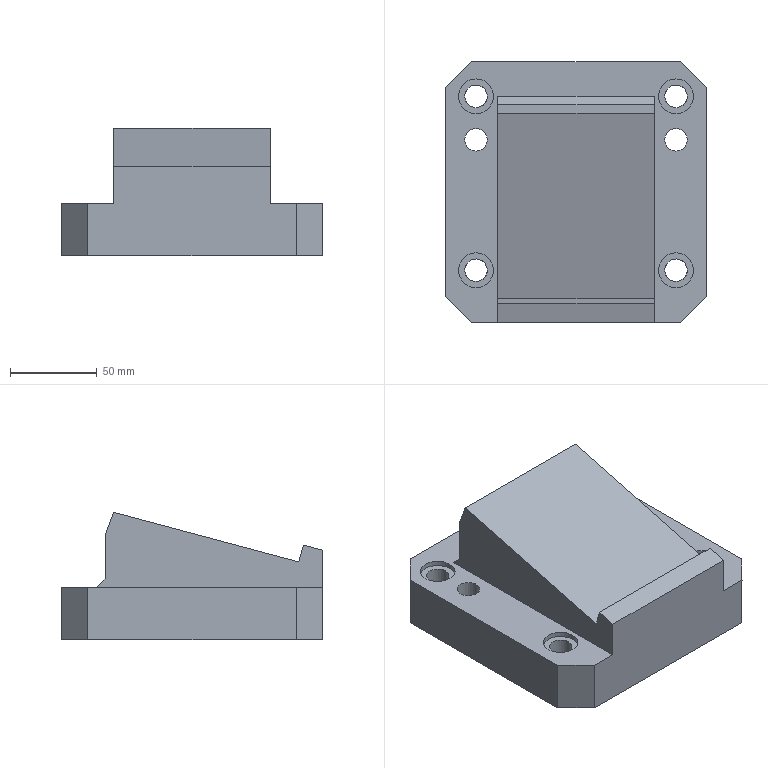Part | NX | features solid 2 | 1 solid | 41 faces | box 150 x 150 x 73.352 mm | volume 930755 mm3 | plane 31 | cylinder 10 | commonest cylinder face diameters 13 x6 20 x4
STEP:
#1=CARTESIAN_POINT('',(227.5,985.,-285.));
#2=VERTEX_POINT('',#1);
#3=CARTESIAN_POINT('',(227.5,995.,-285.));
#4=DIRECTION('',(0.,0.000000003,-1.));
#5=DIRECTION('',(0.,-1.,-0.000000003));
#6=AXIS2_PLACEMENT_3D('',#3,#4,#5);
#7=CIRCLE('',#6,10.);
#8=EDGE_CURVE('',#2,#2,#7,.T.);
#9=ORIENTED_EDGE('',*,*,#8,.T.);
#10=EDGE_LOOP('',(#9));
#11=FACE_BOUND('',#10,.T.);
#12=CARTESIAN_POINT('',(227.5,885.,-285.));
#13=VERTEX_POINT('',#12);
#14=CARTESIAN_POINT('',(227.5,895.,-285.));
#15=DIRECTION('',(0.,0.000000003,-1.));
#16=DIRECTION('',(0.,-1.,-0.000000003));
#17=AXIS2_PLACEMENT_3D('',#14,#15,#16);
#18=CIRCLE('',#17,10.);
#19=EDGE_CURVE('',#13,#13,#18,.T.);
#20=ORIENTED_EDGE('',*,*,#19,.T.);
#21=EDGE_LOOP('',(#20));
#22=FACE_BOUND('',#21,.T.);
#23=CARTESIAN_POINT('',(112.5,963.5,-285.));
#24=VERTEX_POINT('',#23);
#25=CARTESIAN_POINT('',(112.5,970.,-285.));
#26=DIRECTION('',(0.,0.000000003,-1.));
#27=DIRECTION('',(0.,-1.,-0.000000003));
#28=AXIS2_PLACEMENT_3D('',#25,#26,#27);
#29=CIRCLE('',#28,6.5);
#30=EDGE_CURVE('',#24,#24,#29,.T.);
#31=ORIENTED_EDGE('',*,*,#30,.T.);
#32=EDGE_LOOP('',(#31));
#33=FACE_BOUND('',#32,.T.);
#34=CARTESIAN_POINT('',(227.5,963.5,-285.));
#35=VERTEX_POINT('',#34);
#36=CARTESIAN_POINT('',(227.5,970.,-285.));
#37=DIRECTION('',(0.,0.000000003,-1.));
#38=DIRECTION('',(0.,-1.,-0.000000003));
#39=AXIS2_PLACEMENT_3D('',#36,#37,#38);
#40=CIRCLE('',#39,6.5);
#41=EDGE_CURVE('',#35,#35,#40,.T.);
#42=ORIENTED_EDGE('',*,*,#41,.T.);
#43=EDGE_LOOP('',(#42));
#44=FACE_BOUND('',#43,.T.);
#45=CARTESIAN_POINT('',(112.5,885.,-285.));
#46=VERTEX_POINT('',#45);
#47=CARTESIAN_POINT('',(112.5,895.,-285.));
#48=DIRECTION('',(0.,0.000000003,-1.));
#49=DIRECTION('',(0.,-1.,-0.000000003));
#50=AXIS2_PLACEMENT_3D('',#47,#48,#49);
#51=CIRCLE('',#50,10.);
#52=EDGE_CURVE('',#46,#46,#51,.T.);
#53=ORIENTED_EDGE('',*,*,#52,.T.);
#54=EDGE_LOOP('',(#53));
#55=FACE_BOUND('',#54,.T.);
#56=CARTESIAN_POINT('',(112.5,985.,-285.));
#57=VERTEX_POINT('',#56);
#58=CARTESIAN_POINT('',(112.5,995.,-285.));
#59=DIRECTION('',(0.,0.000000003,-1.));
#60=DIRECTION('',(0.,-1.,-0.000000003));
#61=AXIS2_PLACEMENT_3D('',#58,#59,#60);
#62=CIRCLE('',#61,10.);
#63=EDGE_CURVE('',#57,#57,#62,.T.);
#64=ORIENTED_EDGE('',*,*,#63,.T.);
#65=EDGE_LOOP('',(#64));
#66=FACE_BOUND('',#65,.T.);
#67=CARTESIAN_POINT('',(215.,995.,-285.));
#68=VERTEX_POINT('',#67);
#69=CARTESIAN_POINT('',(215.,865.,-285.));
#70=VERTEX_POINT('',#69);
#71=CARTESIAN_POINT('',(215.,990.,-285.));
#72=DIRECTION('',(0.,-1.,-0.000000003));
#73=VECTOR('',#72,1000.);
#74=LINE('',#71,#73);
#75=EDGE_CURVE('',#68,#70,#74,.T.);
#76=ORIENTED_EDGE('',*,*,#75,.T.);
#77=CARTESIAN_POINT('',(230.,865.,-285.));
#78=VERTEX_POINT('',#77);
#79=CARTESIAN_POINT('',(110.,865.,-285.));
#80=DIRECTION('',(1.,0.,0.));
#81=VECTOR('',#80,1000.);
#82=LINE('',#79,#81);
#83=EDGE_CURVE('',#70,#78,#82,.T.);
#84=ORIENTED_EDGE('',*,*,#83,.T.);
#85=CARTESIAN_POINT('',(245.,880.,-285.));
#86=VERTEX_POINT('',#85);
#87=CARTESIAN_POINT('',(245.,880.,-285.));
#88=DIRECTION('',(-0.7071,-0.7071,-0.000000002));
#89=VECTOR('',#88,1000.);
#90=LINE('',#87,#89);
#91=EDGE_CURVE('',#86,#78,#90,.T.);
#92=ORIENTED_EDGE('',*,*,#91,.F.);
#93=CARTESIAN_POINT('',(245.,1000.,-285.));
#94=VERTEX_POINT('',#93);
#95=CARTESIAN_POINT('',(245.,1000.,-285.));
#96=DIRECTION('',(0.,-1.,-0.000000003));
#97=VECTOR('',#96,1000.);
#98=LINE('',#95,#97);
#99=EDGE_CURVE('',#94,#86,#98,.T.);
#100=ORIENTED_EDGE('',*,*,#99,.F.);
#101=CARTESIAN_POINT('',(230.,1015.,-285.));
#102=VERTEX_POINT('',#101);
#103=CARTESIAN_POINT('',(230.,1015.,-285.));
#104=DIRECTION('',(0.7071,-0.7071,-0.000000002));
#105=VECTOR('',#104,1000.);
#106=LINE('',#103,#105);
#107=EDGE_CURVE('',#102,#94,#106,.T.);
#108=ORIENTED_EDGE('',*,*,#107,.F.);
#109=CARTESIAN_POINT('',(110.,1015.,-285.));
#110=VERTEX_POINT('',#109);
#111=CARTESIAN_POINT('',(110.,1015.,-285.));
#112=DIRECTION('',(1.,0.,0.));
#113=VECTOR('',#112,1000.);
#114=LINE('',#111,#113);
#115=EDGE_CURVE('',#110,#102,#114,.T.);
#116=ORIENTED_EDGE('',*,*,#115,.F.);
#117=CARTESIAN_POINT('',(95.,1000.,-285.));
#118=VERTEX_POINT('',#117);
#119=CARTESIAN_POINT('',(95.,1000.,-285.));
#120=DIRECTION('',(0.7071,0.7071,0.000000002));
#121=VECTOR('',#120,1000.);
#122=LINE('',#119,#121);
#123=EDGE_CURVE('',#118,#110,#122,.T.);
#124=ORIENTED_EDGE('',*,*,#123,.F.);
#125=CARTESIAN_POINT('',(95.,880.,-285.));
#126=VERTEX_POINT('',#125);
#127=CARTESIAN_POINT('',(95.,1000.,-285.));
#128=DIRECTION('',(0.,-1.,-0.000000003));
#129=VECTOR('',#128,1000.);
#130=LINE('',#127,#129);
#131=EDGE_CURVE('',#118,#126,#130,.T.);
#132=ORIENTED_EDGE('',*,*,#131,.T.);
#133=CARTESIAN_POINT('',(110.,865.,-285.));
#134=VERTEX_POINT('',#133);
#135=CARTESIAN_POINT('',(110.,865.,-285.));
#136=DIRECTION('',(-0.7071,0.7071,0.000000002));
#137=VECTOR('',#136,1000.);
#138=LINE('',#135,#137);
#139=EDGE_CURVE('',#134,#126,#138,.T.);
#140=ORIENTED_EDGE('',*,*,#139,.F.);
#141=CARTESIAN_POINT('',(125.,865.,-285.));
#142=VERTEX_POINT('',#141);
#143=CARTESIAN_POINT('',(110.,865.,-285.));
#144=DIRECTION('',(1.,0.,0.));
#145=VECTOR('',#144,1000.);
#146=LINE('',#143,#145);
#147=EDGE_CURVE('',#134,#142,#146,.T.);
#148=ORIENTED_EDGE('',*,*,#147,.T.);
#149=CARTESIAN_POINT('',(125.,995.,-285.));
#150=VERTEX_POINT('',#149);
#151=CARTESIAN_POINT('',(125.,990.,-285.));
#152=DIRECTION('',(0.,-1.,-0.000000003));
#153=VECTOR('',#152,1000.);
#154=LINE('',#151,#153);
#155=EDGE_CURVE('',#150,#142,#154,.T.);
#156=ORIENTED_EDGE('',*,*,#155,.F.);
#157=CARTESIAN_POINT('',(170.,995.,-285.));
#158=DIRECTION('',(-1.,0.,0.));
#159=VECTOR('',#158,1000.);
#160=LINE('',#157,#159);
#161=EDGE_CURVE('',#68,#150,#160,.T.);
#162=ORIENTED_EDGE('',*,*,#161,.F.);
#163=EDGE_LOOP('',(#76,#84,#92,#100,#108,#116,#124,#132,#140,#148,#156,#162));
#164=FACE_BOUND('',#163,.T.);
#165=CARTESIAN_POINT('',(170.,805.,-285.));
#166=DIRECTION('',(0.,0.000000003,-1.));
#167=DIRECTION('',(-1.,0.,0.));
#168=AXIS2_PLACEMENT_3D('',#165,#166,#167);
#169=PLANE('',#168);
#170=ADVANCED_FACE('',(#11,#22,#33,#44,#55,#66,#164),#169,.F.);
#171=CARTESIAN_POINT('',(227.5,988.5,-315.));
#172=VERTEX_POINT('',#171);
#173=CARTESIAN_POINT('',(227.5,995.,-315.));
#174=DIRECTION('',(0.,0.000000003,-1.));
#175=DIRECTION('',(0.,-1.,-0.000000003));
#176=AXIS2_PLACEMENT_3D('',#173,#174,#175);
#177=CIRCLE('',#176,6.5);
#178=EDGE_CURVE('',#172,#172,#177,.T.);
#179=ORIENTED_EDGE('',*,*,#178,.T.);
#180=EDGE_LOOP('',(#179));
#181=FACE_BOUND('',#180,.T.);
#182=CARTESIAN_POINT('',(234.,995.,-288.));
#183=VERTEX_POINT('',#182);
#184=CARTESIAN_POINT('',(227.5,995.,-288.));
#185=DIRECTION('',(0.,0.000000003,-1.));
#186=DIRECTION('',(1.,0.,0.));
#187=AXIS2_PLACEMENT_3D('',#184,#185,#186);
#188=CIRCLE('',#187,6.5);
#189=EDGE_CURVE('',#183,#183,#188,.T.);
#190=ORIENTED_EDGE('',*,*,#189,.F.);
#191=EDGE_LOOP('',(#190));
#192=FACE_BOUND('',#191,.T.);
#193=CARTESIAN_POINT('',(227.5,995.,-285.));
#194=DIRECTION('',(0.,0.000000003,-1.));
#195=DIRECTION('',(-1.,0.,0.));
#196=AXIS2_PLACEMENT_3D('',#193,#194,#195);
#197=CYLINDRICAL_SURFACE('',#196,6.5);
#198=ADVANCED_FACE('',(#181,#192),#197,.F.);
#199=CARTESIAN_POINT('',(112.5,988.5,-315.));
#200=VERTEX_POINT('',#199);
#201=CARTESIAN_POINT('',(112.5,995.,-315.));
#202=DIRECTION('',(0.,0.000000003,-1.));
#203=DIRECTION('',(0.,-1.,-0.000000003));
#204=AXIS2_PLACEMENT_3D('',#201,#202,#203);
#205=CIRCLE('',#204,6.5);
#206=EDGE_CURVE('',#200,#200,#205,.T.);
#207=ORIENTED_EDGE('',*,*,#206,.T.);
#208=EDGE_LOOP('',(#207));
#209=FACE_BOUND('',#208,.T.);
#210=CARTESIAN_POINT('',(119.,995.,-288.));
#211=VERTEX_POINT('',#210);
#212=CARTESIAN_POINT('',(112.5,995.,-288.));
#213=DIRECTION('',(0.,0.000000003,-1.));
#214=DIRECTION('',(1.,0.,0.));
#215=AXIS2_PLACEMENT_3D('',#212,#213,#214);
#216=CIRCLE('',#215,6.5);
#217=EDGE_CURVE('',#211,#211,#216,.T.);
#218=ORIENTED_EDGE('',*,*,#217,.F.);
#219=EDGE_LOOP('',(#218));
#220=FACE_BOUND('',#219,.T.);
#221=CARTESIAN_POINT('',(112.5,995.,-285.));
#222=DIRECTION('',(0.,0.000000003,-1.));
#223=DIRECTION('',(-1.,0.,0.));
#224=AXIS2_PLACEMENT_3D('',#221,#222,#223);
#225=CYLINDRICAL_SURFACE('',#224,6.5);
#226=ADVANCED_FACE('',(#209,#220),#225,.F.);
#227=CARTESIAN_POINT('',(227.5,888.5,-315.));
#228=VERTEX_POINT('',#227);
#229=CARTESIAN_POINT('',(227.5,895.,-315.));
#230=DIRECTION('',(0.,0.000000003,-1.));
#231=DIRECTION('',(0.,-1.,-0.000000003));
#232=AXIS2_PLACEMENT_3D('',#229,#230,#231);
#233=CIRCLE('',#232,6.5);
#234=EDGE_CURVE('',#228,#228,#233,.T.);
#235=ORIENTED_EDGE('',*,*,#234,.T.);
#236=EDGE_LOOP('',(#235));
#237=FACE_BOUND('',#236,.T.);
#238=CARTESIAN_POINT('',(234.,895.,-288.));
#239=VERTEX_POINT('',#238);
#240=CARTESIAN_POINT('',(227.5,895.,-288.));
#241=DIRECTION('',(0.,0.000000003,-1.));
#242=DIRECTION('',(1.,0.,0.));
#243=AXIS2_PLACEMENT_3D('',#240,#241,#242);
#244=CIRCLE('',#243,6.5);
#245=EDGE_CURVE('',#239,#239,#244,.T.);
#246=ORIENTED_EDGE('',*,*,#245,.F.);
#247=EDGE_LOOP('',(#246));
#248=FACE_BOUND('',#247,.T.);
#249=CARTESIAN_POINT('',(227.5,895.,-285.));
#250=DIRECTION('',(0.,0.000000003,-1.));
#251=DIRECTION('',(-1.,0.,0.));
#252=AXIS2_PLACEMENT_3D('',#249,#250,#251);
#253=CYLINDRICAL_SURFACE('',#252,6.5);
#254=ADVANCED_FACE('',(#237,#248),#253,.F.);
#255=CARTESIAN_POINT('',(112.5,888.5,-315.));
#256=VERTEX_POINT('',#255);
#257=CARTESIAN_POINT('',(112.5,895.,-315.));
#258=DIRECTION('',(0.,0.000000003,-1.));
#259=DIRECTION('',(0.,-1.,-0.000000003));
#260=AXIS2_PLACEMENT_3D('',#257,#258,#259);
#261=CIRCLE('',#260,6.5);
#262=EDGE_CURVE('',#256,#256,#261,.T.);
#263=ORIENTED_EDGE('',*,*,#262,.T.);
#264=EDGE_LOOP('',(#263));
#265=FACE_BOUND('',#264,.T.);
#266=CARTESIAN_POINT('',(119.,895.,-288.));
#267=VERTEX_POINT('',#266);
#268=CARTESIAN_POINT('',(112.5,895.,-288.));
#269=DIRECTION('',(0.,0.000000003,-1.));
#270=DIRECTION('',(1.,0.,0.));
#271=AXIS2_PLACEMENT_3D('',#268,#269,#270);
#272=CIRCLE('',#271,6.5);
#273=EDGE_CURVE('',#267,#267,#272,.T.);
#274=ORIENTED_EDGE('',*,*,#273,.F.);
#275=EDGE_LOOP('',(#274));
#276=FACE_BOUND('',#275,.T.);
#277=CARTESIAN_POINT('',(112.5,895.,-285.));
#278=DIRECTION('',(0.,0.000000003,-1.));
#279=DIRECTION('',(-1.,0.,0.));
#280=AXIS2_PLACEMENT_3D('',#277,#278,#279);
#281=CYLINDRICAL_SURFACE('',#280,6.5);
#282=ADVANCED_FACE('',(#265,#276),#281,.F.);
#283=CARTESIAN_POINT('',(227.5,963.5,-315.));
#284=VERTEX_POINT('',#283);
#285=CARTESIAN_POINT('',(227.5,970.,-315.));
#286=DIRECTION('',(0.,0.000000003,-1.));
#287=DIRECTION('',(0.,-1.,-0.000000003));
#288=AXIS2_PLACEMENT_3D('',#285,#286,#287);
#289=CIRCLE('',#288,6.5);
#290=EDGE_CURVE('',#284,#284,#289,.T.);
#291=ORIENTED_EDGE('',*,*,#290,.F.);
#292=EDGE_LOOP('',(#291));
#293=FACE_BOUND('',#292,.T.);
#294=ORIENTED_EDGE('',*,*,#206,.F.);
#295=EDGE_LOOP('',(#294));
#296=FACE_BOUND('',#295,.T.);
#297=ORIENTED_EDGE('',*,*,#262,.F.);
#298=EDGE_LOOP('',(#297));
#299=FACE_BOUND('',#298,.T.);
#300=CARTESIAN_POINT('',(110.,865.,-315.));
#301=VERTEX_POINT('',#300);
#302=CARTESIAN_POINT('',(95.,880.,-315.));
#303=VERTEX_POINT('',#302);
#304=CARTESIAN_POINT('',(110.,865.,-315.));
#305=DIRECTION('',(-0.7071,0.7071,0.000000002));
#306=VECTOR('',#305,1000.);
#307=LINE('',#304,#306);
#308=EDGE_CURVE('',#301,#303,#307,.T.);
#309=ORIENTED_EDGE('',*,*,#308,.T.);
#310=CARTESIAN_POINT('',(95.,1000.,-315.));
#311=VERTEX_POINT('',#310);
#312=CARTESIAN_POINT('',(95.,1000.,-315.));
#313=DIRECTION('',(0.,-1.,-0.000000003));
#314=VECTOR('',#313,1000.);
#315=LINE('',#312,#314);
#316=EDGE_CURVE('',#311,#303,#315,.T.);
#317=ORIENTED_EDGE('',*,*,#316,.F.);
#318=CARTESIAN_POINT('',(110.,1015.,-315.));
#319=VERTEX_POINT('',#318);
#320=CARTESIAN_POINT('',(95.,1000.,-315.));
#321=DIRECTION('',(0.7071,0.7071,0.000000002));
#322=VECTOR('',#321,1000.);
#323=LINE('',#320,#322);
#324=EDGE_CURVE('',#311,#319,#323,.T.);
#325=ORIENTED_EDGE('',*,*,#324,.T.);
#326=CARTESIAN_POINT('',(230.,1015.,-315.));
#327=VERTEX_POINT('',#326);
#328=CARTESIAN_POINT('',(110.,1015.,-315.));
#329=DIRECTION('',(1.,0.,0.));
#330=VECTOR('',#329,1000.);
#331=LINE('',#328,#330);
#332=EDGE_CURVE('',#319,#327,#331,.T.);
#333=ORIENTED_EDGE('',*,*,#332,.T.);
#334=CARTESIAN_POINT('',(245.,1000.,-315.));
#335=VERTEX_POINT('',#334);
#336=CARTESIAN_POINT('',(230.,1015.,-315.));
#337=DIRECTION('',(0.7071,-0.7071,-0.000000002));
#338=VECTOR('',#337,1000.);
#339=LINE('',#336,#338);
#340=EDGE_CURVE('',#327,#335,#339,.T.);
#341=ORIENTED_EDGE('',*,*,#340,.T.);
#342=CARTESIAN_POINT('',(245.,880.,-315.));
#343=VERTEX_POINT('',#342);
#344=CARTESIAN_POINT('',(245.,1000.,-315.));
#345=DIRECTION('',(0.,-1.,-0.000000003));
#346=VECTOR('',#345,1000.);
#347=LINE('',#344,#346);
#348=EDGE_CURVE('',#335,#343,#347,.T.);
#349=ORIENTED_EDGE('',*,*,#348,.T.);
#350=CARTESIAN_POINT('',(230.,865.,-315.));
#351=VERTEX_POINT('',#350);
#352=CARTESIAN_POINT('',(245.,880.,-315.));
#353=DIRECTION('',(-0.7071,-0.7071,-0.000000002));
#354=VECTOR('',#353,1000.);
#355=LINE('',#352,#354);
#356=EDGE_CURVE('',#343,#351,#355,.T.);
#357=ORIENTED_EDGE('',*,*,#356,.T.);
#358=CARTESIAN_POINT('',(110.,865.,-315.));
#359=DIRECTION('',(1.,0.,0.));
#360=VECTOR('',#359,1000.);
#361=LINE('',#358,#360);
#362=EDGE_CURVE('',#301,#351,#361,.T.);
#363=ORIENTED_EDGE('',*,*,#362,.F.);
#364=EDGE_LOOP('',(#309,#317,#325,#333,#341,#349,#357,#363));
#365=FACE_BOUND('',#364,.T.);
#366=CARTESIAN_POINT('',(190.,955.,-315.));
#367=VERTEX_POINT('',#366);
#368=CARTESIAN_POINT('',(190.,900.,-315.));
#369=VERTEX_POINT('',#368);
#370=CARTESIAN_POINT('',(190.,955.,-315.));
#371=DIRECTION('',(0.,-1.,-0.000000003));
#372=VECTOR('',#371,1000.);
#373=LINE('',#370,#372);
#374=EDGE_CURVE('',#367,#369,#373,.T.);
#375=ORIENTED_EDGE('',*,*,#374,.F.);
#376=CARTESIAN_POINT('',(180.,965.,-315.));
#377=VERTEX_POINT('',#376);
#378=CARTESIAN_POINT('',(180.,965.,-315.));
#379=DIRECTION('',(0.7071,-0.7071,-0.000000002));
#380=VECTOR('',#379,1000.);
#381=LINE('',#378,#380);
#382=EDGE_CURVE('',#377,#367,#381,.T.);
#383=ORIENTED_EDGE('',*,*,#382,.F.);
#384=CARTESIAN_POINT('',(160.,965.,-315.));
#385=VERTEX_POINT('',#384);
#386=CARTESIAN_POINT('',(160.,965.,-315.));
#387=DIRECTION('',(1.,0.,0.));
#388=VECTOR('',#387,1000.);
#389=LINE('',#386,#388);
#390=EDGE_CURVE('',#385,#377,#389,.T.);
#391=ORIENTED_EDGE('',*,*,#390,.F.);
#392=CARTESIAN_POINT('',(150.,955.,-315.));
#393=VERTEX_POINT('',#392);
#394=CARTESIAN_POINT('',(150.,955.,-315.));
#395=DIRECTION('',(0.7071,0.7071,0.000000002));
#396=VECTOR('',#395,1000.);
#397=LINE('',#394,#396);
#398=EDGE_CURVE('',#393,#385,#397,.T.);
#399=ORIENTED_EDGE('',*,*,#398,.F.);
#400=CARTESIAN_POINT('',(150.,900.,-315.));
#401=VERTEX_POINT('',#400);
#402=CARTESIAN_POINT('',(150.,955.,-315.));
#403=DIRECTION('',(0.,-1.,-0.000000003));
#404=VECTOR('',#403,1000.);
#405=LINE('',#402,#404);
#406=EDGE_CURVE('',#393,#401,#405,.T.);
#407=ORIENTED_EDGE('',*,*,#406,.T.);
#408=CARTESIAN_POINT('',(160.,890.,-315.));
#409=VERTEX_POINT('',#408);
#410=CARTESIAN_POINT('',(160.,890.,-315.));
#411=DIRECTION('',(-0.7071,0.7071,0.000000002));
#412=VECTOR('',#411,1000.);
#413=LINE('',#410,#412);
#414=EDGE_CURVE('',#409,#401,#413,.T.);
#415=ORIENTED_EDGE('',*,*,#414,.F.);
#416=CARTESIAN_POINT('',(180.,890.,-315.));
#417=VERTEX_POINT('',#416);
#418=CARTESIAN_POINT('',(160.,890.,-315.));
#419=DIRECTION('',(1.,0.,0.));
#420=VECTOR('',#419,1000.);
#421=LINE('',#418,#420);
#422=EDGE_CURVE('',#409,#417,#421,.T.);
#423=ORIENTED_EDGE('',*,*,#422,.T.);
#424=CARTESIAN_POINT('',(190.,900.,-315.));
#425=DIRECTION('',(-0.7071,-0.7071,-0.000000002));
#426=VECTOR('',#425,1000.);
#427=LINE('',#424,#426);
#428=EDGE_CURVE('',#369,#417,#427,.T.);
#429=ORIENTED_EDGE('',*,*,#428,.F.);
#430=EDGE_LOOP('',(#375,#383,#391,#399,#407,#415,#423,#429));
#431=FACE_BOUND('',#430,.T.);
#432=ORIENTED_EDGE('',*,*,#234,.F.);
#433=EDGE_LOOP('',(#432));
#434=FACE_BOUND('',#433,.T.);
#435=CARTESIAN_POINT('',(112.5,963.5,-315.));
#436=VERTEX_POINT('',#435);
#437=CARTESIAN_POINT('',(112.5,970.,-315.));
#438=DIRECTION('',(0.,0.000000003,-1.));
#439=DIRECTION('',(0.,-1.,-0.000000003));
#440=AXIS2_PLACEMENT_3D('',#437,#438,#439);
#441=CIRCLE('',#440,6.5);
#442=EDGE_CURVE('',#436,#436,#441,.T.);
#443=ORIENTED_EDGE('',*,*,#442,.F.);
#444=EDGE_LOOP('',(#443));
#445=FACE_BOUND('',#444,.T.);
#446=ORIENTED_EDGE('',*,*,#178,.F.);
#447=EDGE_LOOP('',(#446));
#448=FACE_BOUND('',#447,.T.);
#449=CARTESIAN_POINT('',(170.,805.,-315.));
#450=DIRECTION('',(0.,0.000000003,-1.));
#451=DIRECTION('',(-1.,0.,0.));
#452=AXIS2_PLACEMENT_3D('',#449,#450,#451);
#453=PLANE('',#452);
#454=ADVANCED_FACE('',(#293,#296,#299,#365,#431,#434,#445,#448),#453,.T.);
#455=ORIENTED_EDGE('',*,*,#308,.F.);
#456=CARTESIAN_POINT('',(110.,865.,-285.));
#457=DIRECTION('',(0.,0.000000003,-1.));
#458=VECTOR('',#457,1000.);
#459=LINE('',#456,#458);
#460=EDGE_CURVE('',#134,#301,#459,.T.);
#461=ORIENTED_EDGE('',*,*,#460,.F.);
#462=ORIENTED_EDGE('',*,*,#139,.T.);
#463=CARTESIAN_POINT('',(95.,880.,-285.));
#464=DIRECTION('',(0.,0.000000003,-1.));
#465=VECTOR('',#464,1000.);
#466=LINE('',#463,#465);
#467=EDGE_CURVE('',#126,#303,#466,.T.);
#468=ORIENTED_EDGE('',*,*,#467,.T.);
#469=EDGE_LOOP('',(#455,#461,#462,#468));
#470=FACE_BOUND('',#469,.T.);
#471=CARTESIAN_POINT('',(110.,865.,-285.));
#472=DIRECTION('',(0.7071,0.7071,0.000000002));
#473=DIRECTION('',(0.7071,-0.7071,-0.000000002));
#474=AXIS2_PLACEMENT_3D('',#471,#472,#473);
#475=PLANE('',#474);
#476=ADVANCED_FACE('',(#470),#475,.F.);
#477=ORIENTED_EDGE('',*,*,#316,.T.);
#478=ORIENTED_EDGE('',*,*,#467,.F.);
#479=ORIENTED_EDGE('',*,*,#131,.F.);
#480=CARTESIAN_POINT('',(95.,1000.,-285.));
#481=DIRECTION('',(0.,0.000000003,-1.));
#482=VECTOR('',#481,1000.);
#483=LINE('',#480,#482);
#484=EDGE_CURVE('',#118,#311,#483,.T.);
#485=ORIENTED_EDGE('',*,*,#484,.T.);
#486=EDGE_LOOP('',(#477,#478,#479,#485));
#487=FACE_BOUND('',#486,.T.);
#488=CARTESIAN_POINT('',(95.,1000.,-285.));
#489=DIRECTION('',(-1.,0.,0.));
#490=DIRECTION('',(0.,1.,0.000000003));
#491=AXIS2_PLACEMENT_3D('',#488,#489,#490);
#492=PLANE('',#491);
#493=ADVANCED_FACE('',(#487),#492,.T.);
#494=ORIENTED_EDGE('',*,*,#324,.F.);
#495=ORIENTED_EDGE('',*,*,#484,.F.);
#496=ORIENTED_EDGE('',*,*,#123,.T.);
#497=CARTESIAN_POINT('',(110.,1015.,-285.));
#498=DIRECTION('',(0.,0.000000003,-1.));
#499=VECTOR('',#498,1000.);
#500=LINE('',#497,#499);
#501=EDGE_CURVE('',#110,#319,#500,.T.);
#502=ORIENTED_EDGE('',*,*,#501,.T.);
#503=EDGE_LOOP('',(#494,#495,#496,#502));
#504=FACE_BOUND('',#503,.T.);
#505=CARTESIAN_POINT('',(95.,1000.,-285.));
#506=DIRECTION('',(0.7071,-0.7071,-0.000000002));
#507=DIRECTION('',(-0.7071,-0.7071,-0.000000002));
#508=AXIS2_PLACEMENT_3D('',#505,#506,#507);
#509=PLANE('',#508);
#510=ADVANCED_FACE('',(#504),#509,.F.);
#511=ORIENTED_EDGE('',*,*,#332,.F.);
#512=ORIENTED_EDGE('',*,*,#501,.F.);
#513=ORIENTED_EDGE('',*,*,#115,.T.);
#514=CARTESIAN_POINT('',(230.,1015.,-285.));
#515=DIRECTION('',(0.,0.000000003,-1.));
#516=VECTOR('',#515,1000.);
#517=LINE('',#514,#516);
#518=EDGE_CURVE('',#102,#327,#517,.T.);
#519=ORIENTED_EDGE('',*,*,#518,.T.);
#520=EDGE_LOOP('',(#511,#512,#513,#519));
#521=FACE_BOUND('',#520,.T.);
#522=CARTESIAN_POINT('',(110.,1015.,-285.));
#523=DIRECTION('',(0.,-1.,-0.000000003));
#524=DIRECTION('',(-1.,0.,0.));
#525=AXIS2_PLACEMENT_3D('',#522,#523,#524);
#526=PLANE('',#525);
#527=ADVANCED_FACE('',(#521),#526,.F.);
#528=ORIENTED_EDGE('',*,*,#340,.F.);
#529=ORIENTED_EDGE('',*,*,#518,.F.);
#530=ORIENTED_EDGE('',*,*,#107,.T.);
#531=CARTESIAN_POINT('',(245.,1000.,-285.));
#532=DIRECTION('',(0.,0.000000003,-1.));
#533=VECTOR('',#532,1000.);
#534=LINE('',#531,#533);
#535=EDGE_CURVE('',#94,#335,#534,.T.);
#536=ORIENTED_EDGE('',*,*,#535,.T.);
#537=EDGE_LOOP('',(#528,#529,#530,#536));
#538=FACE_BOUND('',#537,.T.);
#539=CARTESIAN_POINT('',(230.,1015.,-285.));
#540=DIRECTION('',(-0.7071,-0.7071,-0.000000002));
#541=DIRECTION('',(-0.7071,0.7071,0.000000002));
#542=AXIS2_PLACEMENT_3D('',#539,#540,#541);
#543=PLANE('',#542);
#544=ADVANCED_FACE('',(#538),#543,.F.);
#545=ORIENTED_EDGE('',*,*,#348,.F.);
#546=ORIENTED_EDGE('',*,*,#535,.F.);
#547=ORIENTED_EDGE('',*,*,#99,.T.);
#548=CARTESIAN_POINT('',(245.,880.,-285.));
#549=DIRECTION('',(0.,0.000000003,-1.));
#550=VECTOR('',#549,1000.);
#551=LINE('',#548,#550);
#552=EDGE_CURVE('',#86,#343,#551,.T.);
#553=ORIENTED_EDGE('',*,*,#552,.T.);
#554=EDGE_LOOP('',(#545,#546,#547,#553));
#555=FACE_BOUND('',#554,.T.);
#556=CARTESIAN_POINT('',(245.,1000.,-285.));
#557=DIRECTION('',(-1.,0.,0.));
#558=DIRECTION('',(0.,1.,0.000000003));
#559=AXIS2_PLACEMENT_3D('',#556,#557,#558);
#560=PLANE('',#559);
#561=ADVANCED_FACE('',(#555),#560,.F.);
#562=ORIENTED_EDGE('',*,*,#356,.F.);
#563=ORIENTED_EDGE('',*,*,#552,.F.);
#564=ORIENTED_EDGE('',*,*,#91,.T.);
#565=CARTESIAN_POINT('',(230.,865.,-285.));
#566=DIRECTION('',(0.,0.000000003,-1.));
#567=VECTOR('',#566,1000.);
#568=LINE('',#565,#567);
#569=EDGE_CURVE('',#78,#351,#568,.T.);
#570=ORIENTED_EDGE('',*,*,#569,.T.);
#571=EDGE_LOOP('',(#562,#563,#564,#570));
#572=FACE_BOUND('',#571,.T.);
#573=CARTESIAN_POINT('',(245.,880.,-285.));
#574=DIRECTION('',(-0.7071,0.7071,0.000000002));
#575=DIRECTION('',(0.7071,0.7071,0.000000002));
#576=AXIS2_PLACEMENT_3D('',#573,#574,#575);
#577=PLANE('',#576);
#578=ADVANCED_FACE('',(#572),#577,.F.);
#579=ORIENTED_EDGE('',*,*,#362,.T.);
#580=ORIENTED_EDGE('',*,*,#569,.F.);
#581=ORIENTED_EDGE('',*,*,#83,.F.);
#582=CARTESIAN_POINT('',(215.,865.,-263.487));
#583=VERTEX_POINT('',#582);
#584=CARTESIAN_POINT('',(215.,865.,-285.));
#585=DIRECTION('',(0.,-0.000000003,1.));
#586=VECTOR('',#585,1000.);
#587=LINE('',#584,#586);
#588=EDGE_CURVE('',#70,#583,#587,.T.);
#589=ORIENTED_EDGE('',*,*,#588,.T.);
#590=CARTESIAN_POINT('',(125.,865.,-263.487));
#591=VERTEX_POINT('',#590);
#592=CARTESIAN_POINT('',(125.,865.,-263.487));
#593=DIRECTION('',(1.,0.,0.));
#594=VECTOR('',#593,1000.);
#595=LINE('',#592,#594);
#596=EDGE_CURVE('',#591,#583,#595,.T.);
#597=ORIENTED_EDGE('',*,*,#596,.F.);
#598=CARTESIAN_POINT('',(125.,865.,-285.));
#599=DIRECTION('',(0.,-0.000000003,1.));
#600=VECTOR('',#599,1000.);
#601=LINE('',#598,#600);
#602=EDGE_CURVE('',#142,#591,#601,.T.);
#603=ORIENTED_EDGE('',*,*,#602,.F.);
#604=ORIENTED_EDGE('',*,*,#147,.F.);
#605=ORIENTED_EDGE('',*,*,#460,.T.);
#606=EDGE_LOOP('',(#579,#580,#581,#589,#597,#603,#604,#605));
#607=FACE_BOUND('',#606,.T.);
#608=CARTESIAN_POINT('',(110.,865.,-285.));
#609=DIRECTION('',(0.,-1.,-0.000000003));
#610=DIRECTION('',(-1.,0.,0.));
#611=AXIS2_PLACEMENT_3D('',#608,#609,#610);
#612=PLANE('',#611);
#613=ADVANCED_FACE('',(#607),#612,.T.);
#614=ORIENTED_EDGE('',*,*,#428,.T.);
#615=CARTESIAN_POINT('',(180.,890.,-305.));
#616=VERTEX_POINT('',#615);
#617=CARTESIAN_POINT('',(180.,890.,-305.));
#618=DIRECTION('',(0.,0.000000003,-1.));
#619=VECTOR('',#618,1000.);
#620=LINE('',#617,#619);
#621=EDGE_CURVE('',#616,#417,#620,.T.);
#622=ORIENTED_EDGE('',*,*,#621,.F.);
#623=CARTESIAN_POINT('',(190.,900.,-305.));
#624=VERTEX_POINT('',#623);
#625=CARTESIAN_POINT('',(190.,900.,-305.));
#626=DIRECTION('',(-0.7071,-0.7071,-0.000000002));
#627=VECTOR('',#626,1000.);
#628=LINE('',#625,#627);
#629=EDGE_CURVE('',#624,#616,#628,.T.);
#630=ORIENTED_EDGE('',*,*,#629,.F.);
#631=CARTESIAN_POINT('',(190.,900.,-305.));
#632=DIRECTION('',(0.,0.000000003,-1.));
#633=VECTOR('',#632,1000.);
#634=LINE('',#631,#633);
#635=EDGE_CURVE('',#624,#369,#634,.T.);
#636=ORIENTED_EDGE('',*,*,#635,.T.);
#637=EDGE_LOOP('',(#614,#622,#630,#636));
#638=FACE_BOUND('',#637,.T.);
#639=CARTESIAN_POINT('',(190.,900.,-305.));
#640=DIRECTION('',(-0.7071,0.7071,0.000000002));
#641=DIRECTION('',(0.7071,0.7071,0.000000002));
#642=AXIS2_PLACEMENT_3D('',#639,#640,#641);
#643=PLANE('',#642);
#644=ADVANCED_FACE('',(#638),#643,.T.);
#645=ORIENTED_EDGE('',*,*,#422,.F.);
#646=CARTESIAN_POINT('',(160.,890.,-305.));
#647=VERTEX_POINT('',#646);
#648=CARTESIAN_POINT('',(160.,890.,-305.));
#649=DIRECTION('',(0.,0.000000003,-1.));
#650=VECTOR('',#649,1000.);
#651=LINE('',#648,#650);
#652=EDGE_CURVE('',#647,#409,#651,.T.);
#653=ORIENTED_EDGE('',*,*,#652,.F.);
#654=CARTESIAN_POINT('',(160.,890.,-305.));
#655=DIRECTION('',(1.,0.,0.));
#656=VECTOR('',#655,1000.);
#657=LINE('',#654,#656);
#658=EDGE_CURVE('',#647,#616,#657,.T.);
#659=ORIENTED_EDGE('',*,*,#658,.T.);
#660=ORIENTED_EDGE('',*,*,#621,.T.);
#661=EDGE_LOOP('',(#645,#653,#659,#660));
#662=FACE_BOUND('',#661,.T.);
#663=CARTESIAN_POINT('',(160.,890.,-305.));
#664=DIRECTION('',(0.,-1.,-0.000000003));
#665=DIRECTION('',(-1.,0.,0.));
#666=AXIS2_PLACEMENT_3D('',#663,#664,#665);
#667=PLANE('',#666);
#668=ADVANCED_FACE('',(#662),#667,.F.);
#669=ORIENTED_EDGE('',*,*,#414,.T.);
#670=CARTESIAN_POINT('',(150.,900.,-305.));
#671=VERTEX_POINT('',#670);
#672=CARTESIAN_POINT('',(150.,900.,-305.));
#673=DIRECTION('',(0.,0.000000003,-1.));
#674=VECTOR('',#673,1000.);
#675=LINE('',#672,#674);
#676=EDGE_CURVE('',#671,#401,#675,.T.);
#677=ORIENTED_EDGE('',*,*,#676,.F.);
#678=CARTESIAN_POINT('',(160.,890.,-305.));
#679=DIRECTION('',(-0.7071,0.7071,0.000000002));
#680=VECTOR('',#679,1000.);
#681=LINE('',#678,#680);
#682=EDGE_CURVE('',#647,#671,#681,.T.);
#683=ORIENTED_EDGE('',*,*,#682,.F.);
#684=ORIENTED_EDGE('',*,*,#652,.T.);
#685=EDGE_LOOP('',(#669,#677,#683,#684));
#686=FACE_BOUND('',#685,.T.);
#687=CARTESIAN_POINT('',(160.,890.,-305.));
#688=DIRECTION('',(0.7071,0.7071,0.000000002));
#689=DIRECTION('',(0.7071,-0.7071,-0.000000002));
#690=AXIS2_PLACEMENT_3D('',#687,#688,#689);
#691=PLANE('',#690);
#692=ADVANCED_FACE('',(#686),#691,.T.);
#693=ORIENTED_EDGE('',*,*,#406,.F.);
#694=CARTESIAN_POINT('',(150.,955.,-305.));
#695=VERTEX_POINT('',#694);
#696=CARTESIAN_POINT('',(150.,955.,-305.));
#697=DIRECTION('',(0.,0.000000003,-1.));
#698=VECTOR('',#697,1000.);
#699=LINE('',#696,#698);
#700=EDGE_CURVE('',#695,#393,#699,.T.);
#701=ORIENTED_EDGE('',*,*,#700,.F.);
#702=CARTESIAN_POINT('',(150.,955.,-305.));
#703=DIRECTION('',(0.,-1.,-0.000000003));
#704=VECTOR('',#703,1000.);
#705=LINE('',#702,#704);
#706=EDGE_CURVE('',#695,#671,#705,.T.);
#707=ORIENTED_EDGE('',*,*,#706,.T.);
#708=ORIENTED_EDGE('',*,*,#676,.T.);
#709=EDGE_LOOP('',(#693,#701,#707,#708));
#710=FACE_BOUND('',#709,.T.);
#711=CARTESIAN_POINT('',(150.,955.,-305.));
#712=DIRECTION('',(-1.,0.,0.));
#713=DIRECTION('',(0.,1.,0.000000003));
#714=AXIS2_PLACEMENT_3D('',#711,#712,#713);
#715=PLANE('',#714);
#716=ADVANCED_FACE('',(#710),#715,.F.);
#717=ORIENTED_EDGE('',*,*,#398,.T.);
#718=CARTESIAN_POINT('',(160.,965.,-305.));
#719=VERTEX_POINT('',#718);
#720=CARTESIAN_POINT('',(160.,965.,-305.));
#721=DIRECTION('',(0.,0.000000003,-1.));
#722=VECTOR('',#721,1000.);
#723=LINE('',#720,#722);
#724=EDGE_CURVE('',#719,#385,#723,.T.);
#725=ORIENTED_EDGE('',*,*,#724,.F.);
#726=CARTESIAN_POINT('',(150.,955.,-305.));
#727=DIRECTION('',(0.7071,0.7071,0.000000002));
#728=VECTOR('',#727,1000.);
#729=LINE('',#726,#728);
#730=EDGE_CURVE('',#695,#719,#729,.T.);
#731=ORIENTED_EDGE('',*,*,#730,.F.);
#732=ORIENTED_EDGE('',*,*,#700,.T.);
#733=EDGE_LOOP('',(#717,#725,#731,#732));
#734=FACE_BOUND('',#733,.T.);
#735=CARTESIAN_POINT('',(150.,955.,-305.));
#736=DIRECTION('',(0.7071,-0.7071,-0.000000002));
#737=DIRECTION('',(-0.7071,-0.7071,-0.000000002));
#738=AXIS2_PLACEMENT_3D('',#735,#736,#737);
#739=PLANE('',#738);
#740=ADVANCED_FACE('',(#734),#739,.T.);
#741=ORIENTED_EDGE('',*,*,#390,.T.);
#742=CARTESIAN_POINT('',(180.,965.,-305.));
#743=VERTEX_POINT('',#742);
#744=CARTESIAN_POINT('',(180.,965.,-305.));
#745=DIRECTION('',(0.,0.000000003,-1.));
#746=VECTOR('',#745,1000.);
#747=LINE('',#744,#746);
#748=EDGE_CURVE('',#743,#377,#747,.T.);
#749=ORIENTED_EDGE('',*,*,#748,.F.);
#750=CARTESIAN_POINT('',(160.,965.,-305.));
#751=DIRECTION('',(1.,0.,0.));
#752=VECTOR('',#751,1000.);
#753=LINE('',#750,#752);
#754=EDGE_CURVE('',#719,#743,#753,.T.);
#755=ORIENTED_EDGE('',*,*,#754,.F.);
#756=ORIENTED_EDGE('',*,*,#724,.T.);
#757=EDGE_LOOP('',(#741,#749,#755,#756));
#758=FACE_BOUND('',#757,.T.);
#759=CARTESIAN_POINT('',(160.,965.,-305.));
#760=DIRECTION('',(0.,-1.,-0.000000003));
#761=DIRECTION('',(-1.,0.,0.));
#762=AXIS2_PLACEMENT_3D('',#759,#760,#761);
#763=PLANE('',#762);
#764=ADVANCED_FACE('',(#758),#763,.T.);
#765=ORIENTED_EDGE('',*,*,#382,.T.);
#766=CARTESIAN_POINT('',(190.,955.,-305.));
#767=VERTEX_POINT('',#766);
#768=CARTESIAN_POINT('',(190.,955.,-305.));
#769=DIRECTION('',(0.,0.000000003,-1.));
#770=VECTOR('',#769,1000.);
#771=LINE('',#768,#770);
#772=EDGE_CURVE('',#767,#367,#771,.T.);
#773=ORIENTED_EDGE('',*,*,#772,.F.);
#774=CARTESIAN_POINT('',(180.,965.,-305.));
#775=DIRECTION('',(0.7071,-0.7071,-0.000000002));
#776=VECTOR('',#775,1000.);
#777=LINE('',#774,#776);
#778=EDGE_CURVE('',#743,#767,#777,.T.);
#779=ORIENTED_EDGE('',*,*,#778,.F.);
#780=ORIENTED_EDGE('',*,*,#748,.T.);
#781=EDGE_LOOP('',(#765,#773,#779,#780));
#782=FACE_BOUND('',#781,.T.);
#783=CARTESIAN_POINT('',(180.,965.,-305.));
#784=DIRECTION('',(-0.7071,-0.7071,-0.000000002));
#785=DIRECTION('',(-0.7071,0.7071,0.000000002));
#786=AXIS2_PLACEMENT_3D('',#783,#784,#785);
#787=PLANE('',#786);
#788=ADVANCED_FACE('',(#782),#787,.T.);
#789=ORIENTED_EDGE('',*,*,#374,.T.);
#790=ORIENTED_EDGE('',*,*,#635,.F.);
#791=CARTESIAN_POINT('',(190.,955.,-305.));
#792=DIRECTION('',(0.,-1.,-0.000000003));
#793=VECTOR('',#792,1000.);
#794=LINE('',#791,#793);
#795=EDGE_CURVE('',#767,#624,#794,.T.);
#796=ORIENTED_EDGE('',*,*,#795,.F.);
#797=ORIENTED_EDGE('',*,*,#772,.T.);
#798=EDGE_LOOP('',(#789,#790,#796,#797));
#799=FACE_BOUND('',#798,.T.);
#800=CARTESIAN_POINT('',(190.,955.,-305.));
#801=DIRECTION('',(-1.,0.,0.));
#802=DIRECTION('',(0.,1.,0.000000003));
#803=AXIS2_PLACEMENT_3D('',#800,#801,#802);
#804=PLANE('',#803);
#805=ADVANCED_FACE('',(#799),#804,.T.);
#806=ORIENTED_EDGE('',*,*,#629,.T.);
#807=ORIENTED_EDGE('',*,*,#658,.F.);
#808=ORIENTED_EDGE('',*,*,#682,.T.);
#809=ORIENTED_EDGE('',*,*,#706,.F.);
#810=ORIENTED_EDGE('',*,*,#730,.T.);
#811=ORIENTED_EDGE('',*,*,#754,.T.);
#812=ORIENTED_EDGE('',*,*,#778,.T.);
#813=ORIENTED_EDGE('',*,*,#795,.T.);
#814=EDGE_LOOP('',(#806,#807,#808,#809,#810,#811,#812,#813));
#815=FACE_BOUND('',#814,.T.);
#816=CARTESIAN_POINT('',(170.,880.,-305.));
#817=DIRECTION('',(0.,-0.000000003,1.));
#818=DIRECTION('',(1.,0.,0.));
#819=AXIS2_PLACEMENT_3D('',#816,#817,#818);
#820=PLANE('',#819);
#821=ADVANCED_FACE('',(#815),#820,.F.);
#822=ORIENTED_EDGE('',*,*,#30,.F.);
#823=EDGE_LOOP('',(#822));
#824=FACE_BOUND('',#823,.T.);
#825=ORIENTED_EDGE('',*,*,#442,.T.);
#826=EDGE_LOOP('',(#825));
#827=FACE_BOUND('',#826,.T.);
#828=CARTESIAN_POINT('',(112.5,970.,-285.));
#829=DIRECTION('',(0.,0.000000003,-1.));
#830=DIRECTION('',(-1.,0.,0.));
#831=AXIS2_PLACEMENT_3D('',#828,#829,#830);
#832=CYLINDRICAL_SURFACE('',#831,6.5);
#833=ADVANCED_FACE('',(#824,#827),#832,.F.);
#834=ORIENTED_EDGE('',*,*,#41,.F.);
#835=EDGE_LOOP('',(#834));
#836=FACE_BOUND('',#835,.T.);
#837=ORIENTED_EDGE('',*,*,#290,.T.);
#838=EDGE_LOOP('',(#837));
#839=FACE_BOUND('',#838,.T.);
#840=CARTESIAN_POINT('',(227.5,970.,-285.));
#841=DIRECTION('',(0.,0.000000003,-1.));
#842=DIRECTION('',(-1.,0.,0.));
#843=AXIS2_PLACEMENT_3D('',#840,#841,#842);
#844=CYLINDRICAL_SURFACE('',#843,6.5);
#845=ADVANCED_FACE('',(#836,#839),#844,.F.);
#846=ORIENTED_EDGE('',*,*,#52,.F.);
#847=EDGE_LOOP('',(#846));
#848=FACE_BOUND('',#847,.T.);
#849=CARTESIAN_POINT('',(112.5,885.,-288.));
#850=VERTEX_POINT('',#849);
#851=CARTESIAN_POINT('',(112.5,895.,-288.));
#852=DIRECTION('',(0.,0.000000003,-1.));
#853=DIRECTION('',(0.,-1.,-0.000000003));
#854=AXIS2_PLACEMENT_3D('',#851,#852,#853);
#855=CIRCLE('',#854,10.);
#856=EDGE_CURVE('',#850,#850,#855,.T.);
#857=ORIENTED_EDGE('',*,*,#856,.T.);
#858=EDGE_LOOP('',(#857));
#859=FACE_BOUND('',#858,.T.);
#860=CARTESIAN_POINT('',(112.5,895.,-285.));
#861=DIRECTION('',(0.,0.000000003,-1.));
#862=DIRECTION('',(-1.,0.,0.));
#863=AXIS2_PLACEMENT_3D('',#860,#861,#862);
#864=CYLINDRICAL_SURFACE('',#863,10.);
#865=ADVANCED_FACE('',(#848,#859),#864,.F.);
#866=ORIENTED_EDGE('',*,*,#273,.T.);
#867=EDGE_LOOP('',(#866));
#868=FACE_BOUND('',#867,.T.);
#869=ORIENTED_EDGE('',*,*,#856,.F.);
#870=EDGE_LOOP('',(#869));
#871=FACE_BOUND('',#870,.T.);
#872=CARTESIAN_POINT('',(112.5,895.,-288.));
#873=DIRECTION('',(0.,-0.000000003,1.));
#874=DIRECTION('',(1.,0.,0.));
#875=AXIS2_PLACEMENT_3D('',#872,#873,#874);
#876=PLANE('',#875);
#877=ADVANCED_FACE('',(#868,#871),#876,.T.);
#878=ORIENTED_EDGE('',*,*,#19,.F.);
#879=EDGE_LOOP('',(#878));
#880=FACE_BOUND('',#879,.T.);
#881=CARTESIAN_POINT('',(227.5,885.,-288.));
#882=VERTEX_POINT('',#881);
#883=CARTESIAN_POINT('',(227.5,895.,-288.));
#884=DIRECTION('',(0.,0.000000003,-1.));
#885=DIRECTION('',(0.,-1.,-0.000000003));
#886=AXIS2_PLACEMENT_3D('',#883,#884,#885);
#887=CIRCLE('',#886,10.);
#888=EDGE_CURVE('',#882,#882,#887,.T.);
#889=ORIENTED_EDGE('',*,*,#888,.T.);
#890=EDGE_LOOP('',(#889));
#891=FACE_BOUND('',#890,.T.);
#892=CARTESIAN_POINT('',(227.5,895.,-285.));
#893=DIRECTION('',(0.,0.000000003,-1.));
#894=DIRECTION('',(-1.,0.,0.));
#895=AXIS2_PLACEMENT_3D('',#892,#893,#894);
#896=CYLINDRICAL_SURFACE('',#895,10.);
#897=ADVANCED_FACE('',(#880,#891),#896,.F.);
#898=ORIENTED_EDGE('',*,*,#245,.T.);
#899=EDGE_LOOP('',(#898));
#900=FACE_BOUND('',#899,.T.);
#901=ORIENTED_EDGE('',*,*,#888,.F.);
#902=EDGE_LOOP('',(#901));
#903=FACE_BOUND('',#902,.T.);
#904=CARTESIAN_POINT('',(227.5,895.,-288.));
#905=DIRECTION('',(0.,-0.000000003,1.));
#906=DIRECTION('',(1.,0.,0.));
#907=AXIS2_PLACEMENT_3D('',#904,#905,#906);
#908=PLANE('',#907);
#909=ADVANCED_FACE('',(#900,#903),#908,.T.);
#910=ORIENTED_EDGE('',*,*,#63,.F.);
#911=EDGE_LOOP('',(#910));
#912=FACE_BOUND('',#911,.T.);
#913=CARTESIAN_POINT('',(112.5,985.,-288.));
#914=VERTEX_POINT('',#913);
#915=CARTESIAN_POINT('',(112.5,995.,-288.));
#916=DIRECTION('',(0.,0.000000003,-1.));
#917=DIRECTION('',(0.,-1.,-0.000000003));
#918=AXIS2_PLACEMENT_3D('',#915,#916,#917);
#919=CIRCLE('',#918,10.);
#920=EDGE_CURVE('',#914,#914,#919,.T.);
#921=ORIENTED_EDGE('',*,*,#920,.T.);
#922=EDGE_LOOP('',(#921));
#923=FACE_BOUND('',#922,.T.);
#924=CARTESIAN_POINT('',(112.5,995.,-285.));
#925=DIRECTION('',(0.,0.000000003,-1.));
#926=DIRECTION('',(-1.,0.,0.));
#927=AXIS2_PLACEMENT_3D('',#924,#925,#926);
#928=CYLINDRICAL_SURFACE('',#927,10.);
#929=ADVANCED_FACE('',(#912,#923),#928,.F.);
#930=ORIENTED_EDGE('',*,*,#217,.T.);
#931=EDGE_LOOP('',(#930));
#932=FACE_BOUND('',#931,.T.);
#933=ORIENTED_EDGE('',*,*,#920,.F.);
#934=EDGE_LOOP('',(#933));
#935=FACE_BOUND('',#934,.T.);
#936=CARTESIAN_POINT('',(112.5,995.,-288.));
#937=DIRECTION('',(0.,-0.000000003,1.));
#938=DIRECTION('',(1.,0.,0.));
#939=AXIS2_PLACEMENT_3D('',#936,#937,#938);
#940=PLANE('',#939);
#941=ADVANCED_FACE('',(#932,#935),#940,.T.);
#942=ORIENTED_EDGE('',*,*,#8,.F.);
#943=EDGE_LOOP('',(#942));
#944=FACE_BOUND('',#943,.T.);
#945=CARTESIAN_POINT('',(227.5,985.,-288.));
#946=VERTEX_POINT('',#945);
#947=CARTESIAN_POINT('',(227.5,995.,-288.));
#948=DIRECTION('',(0.,0.000000003,-1.));
#949=DIRECTION('',(0.,-1.,-0.000000003));
#950=AXIS2_PLACEMENT_3D('',#947,#948,#949);
#951=CIRCLE('',#950,10.);
#952=EDGE_CURVE('',#946,#946,#951,.T.);
#953=ORIENTED_EDGE('',*,*,#952,.T.);
#954=EDGE_LOOP('',(#953));
#955=FACE_BOUND('',#954,.T.);
#956=CARTESIAN_POINT('',(227.5,995.,-285.));
#957=DIRECTION('',(0.,0.000000003,-1.));
#958=DIRECTION('',(-1.,0.,0.));
#959=AXIS2_PLACEMENT_3D('',#956,#957,#958);
#960=CYLINDRICAL_SURFACE('',#959,10.);
#961=ADVANCED_FACE('',(#944,#955),#960,.F.);
#962=ORIENTED_EDGE('',*,*,#189,.T.);
#963=EDGE_LOOP('',(#962));
#964=FACE_BOUND('',#963,.T.);
#965=ORIENTED_EDGE('',*,*,#952,.F.);
#966=EDGE_LOOP('',(#965));
#967=FACE_BOUND('',#966,.T.);
#968=CARTESIAN_POINT('',(227.5,995.,-288.));
#969=DIRECTION('',(0.,-0.000000003,1.));
#970=DIRECTION('',(1.,0.,0.));
#971=AXIS2_PLACEMENT_3D('',#968,#969,#970);
#972=PLANE('',#971);
#973=ADVANCED_FACE('',(#964,#967),#972,.T.);
#974=CARTESIAN_POINT('',(215.,985.14,-241.648));
#975=VERTEX_POINT('',#974);
#976=CARTESIAN_POINT('',(215.,878.584,-270.2));
#977=VERTEX_POINT('',#976);
#978=CARTESIAN_POINT('',(215.,985.14,-241.648));
#979=DIRECTION('',(0.,-0.9659,-0.2588));
#980=VECTOR('',#979,1000.);
#981=LINE('',#978,#980);
#982=EDGE_CURVE('',#975,#977,#981,.T.);
#983=ORIENTED_EDGE('',*,*,#982,.F.);
#984=CARTESIAN_POINT('',(125.,985.14,-241.648));
#985=VERTEX_POINT('',#984);
#986=CARTESIAN_POINT('',(125.,985.14,-241.648));
#987=DIRECTION('',(1.,0.,0.));
#988=VECTOR('',#987,1000.);
#989=LINE('',#986,#988);
#990=EDGE_CURVE('',#985,#975,#989,.T.);
#991=ORIENTED_EDGE('',*,*,#990,.F.);
#992=CARTESIAN_POINT('',(125.,878.584,-270.2));
#993=VERTEX_POINT('',#992);
#994=CARTESIAN_POINT('',(125.,985.14,-241.648));
#995=DIRECTION('',(0.,-0.9659,-0.2588));
#996=VECTOR('',#995,1000.);
#997=LINE('',#994,#996);
#998=EDGE_CURVE('',#985,#993,#997,.T.);
#999=ORIENTED_EDGE('',*,*,#998,.T.);
#1000=CARTESIAN_POINT('',(125.,878.584,-270.2));
#1001=DIRECTION('',(1.,0.,0.));
#1002=VECTOR('',#1001,1000.);
#1003=LINE('',#1000,#1002);
#1004=EDGE_CURVE('',#993,#977,#1003,.T.);
#1005=ORIENTED_EDGE('',*,*,#1004,.T.);
#1006=EDGE_LOOP('',(#983,#991,#999,#1005));
#1007=FACE_BOUND('',#1006,.T.);
#1008=CARTESIAN_POINT('',(125.,985.14,-241.648));
#1009=DIRECTION('',(0.,0.2588,-0.9659));
#1010=DIRECTION('',(0.,-0.9659,-0.2588));
#1011=AXIS2_PLACEMENT_3D('',#1008,#1009,#1010);
#1012=PLANE('',#1011);
#1013=ADVANCED_FACE('',(#1007),#1012,.F.);
#1014=CARTESIAN_POINT('',(215.,875.996,-260.541));
#1015=VERTEX_POINT('',#1014);
#1016=CARTESIAN_POINT('',(215.,878.584,-270.2));
#1017=DIRECTION('',(0.,-0.2588,0.9659));
#1018=VECTOR('',#1017,1000.);
#1019=LINE('',#1016,#1018);
#1020=EDGE_CURVE('',#977,#1015,#1019,.T.);
#1021=ORIENTED_EDGE('',*,*,#1020,.F.);
#1022=ORIENTED_EDGE('',*,*,#1004,.F.);
#1023=CARTESIAN_POINT('',(125.,875.996,-260.541));
#1024=VERTEX_POINT('',#1023);
#1025=CARTESIAN_POINT('',(125.,878.584,-270.2));
#1026=DIRECTION('',(0.,-0.2588,0.9659));
#1027=VECTOR('',#1026,1000.);
#1028=LINE('',#1025,#1027);
#1029=EDGE_CURVE('',#993,#1024,#1028,.T.);
#1030=ORIENTED_EDGE('',*,*,#1029,.T.);
#1031=CARTESIAN_POINT('',(125.,875.996,-260.541));
#1032=DIRECTION('',(1.,0.,0.));
#1033=VECTOR('',#1032,1000.);
#1034=LINE('',#1031,#1033);
#1035=EDGE_CURVE('',#1024,#1015,#1034,.T.);
#1036=ORIENTED_EDGE('',*,*,#1035,.T.);
#1037=EDGE_LOOP('',(#1021,#1022,#1030,#1036));
#1038=FACE_BOUND('',#1037,.T.);
#1039=CARTESIAN_POINT('',(125.,878.584,-270.2));
#1040=DIRECTION('',(0.,-0.9659,-0.2588));
#1041=DIRECTION('',(0.,-0.2588,0.9659));
#1042=AXIS2_PLACEMENT_3D('',#1039,#1040,#1041);
#1043=PLANE('',#1042);
#1044=ADVANCED_FACE('',(#1038),#1043,.F.);
#1045=CARTESIAN_POINT('',(215.,875.996,-260.541));
#1046=DIRECTION('',(0.,-0.9659,-0.2588));
#1047=VECTOR('',#1046,1000.);
#1048=LINE('',#1045,#1047);
#1049=EDGE_CURVE('',#1015,#583,#1048,.T.);
#1050=ORIENTED_EDGE('',*,*,#1049,.F.);
#1051=ORIENTED_EDGE('',*,*,#1035,.F.);
#1052=CARTESIAN_POINT('',(125.,875.996,-260.541));
#1053=DIRECTION('',(0.,-0.9659,-0.2588));
#1054=VECTOR('',#1053,1000.);
#1055=LINE('',#1052,#1054);
#1056=EDGE_CURVE('',#1024,#591,#1055,.T.);
#1057=ORIENTED_EDGE('',*,*,#1056,.T.);
#1058=ORIENTED_EDGE('',*,*,#596,.T.);
#1059=EDGE_LOOP('',(#1050,#1051,#1057,#1058));
#1060=FACE_BOUND('',#1059,.T.);
#1061=CARTESIAN_POINT('',(125.,875.996,-260.541));
#1062=DIRECTION('',(0.,0.2588,-0.9659));
#1063=DIRECTION('',(0.,-0.9659,-0.2588));
#1064=AXIS2_PLACEMENT_3D('',#1061,#1062,#1063);
#1065=PLANE('',#1064);
#1066=ADVANCED_FACE('',(#1060),#1065,.F.);
#1067=CARTESIAN_POINT('',(125.,990.,-255.));
#1068=VERTEX_POINT('',#1067);
#1069=CARTESIAN_POINT('',(125.,990.,-280.));
#1070=VERTEX_POINT('',#1069);
#1071=CARTESIAN_POINT('',(125.,990.,-255.));
#1072=DIRECTION('',(0.,0.000000003,-1.));
#1073=VECTOR('',#1072,1000.);
#1074=LINE('',#1071,#1073);
#1075=EDGE_CURVE('',#1068,#1070,#1074,.T.);
#1076=ORIENTED_EDGE('',*,*,#1075,.F.);
#1077=CARTESIAN_POINT('',(215.,990.,-255.));
#1078=VERTEX_POINT('',#1077);
#1079=CARTESIAN_POINT('',(125.,990.,-255.));
#1080=DIRECTION('',(1.,0.,0.));
#1081=VECTOR('',#1080,1000.);
#1082=LINE('',#1079,#1081);
#1083=EDGE_CURVE('',#1068,#1078,#1082,.T.);
#1084=ORIENTED_EDGE('',*,*,#1083,.T.);
#1085=CARTESIAN_POINT('',(215.,990.,-280.));
#1086=VERTEX_POINT('',#1085);
#1087=CARTESIAN_POINT('',(215.,990.,-255.));
#1088=DIRECTION('',(0.,0.000000003,-1.));
#1089=VECTOR('',#1088,1000.);
#1090=LINE('',#1087,#1089);
#1091=EDGE_CURVE('',#1078,#1086,#1090,.T.);
#1092=ORIENTED_EDGE('',*,*,#1091,.T.);
#1093=CARTESIAN_POINT('',(125.,990.,-280.));
#1094=DIRECTION('',(1.,0.,0.));
#1095=VECTOR('',#1094,1000.);
#1096=LINE('',#1093,#1095);
#1097=EDGE_CURVE('',#1070,#1086,#1096,.T.);
#1098=ORIENTED_EDGE('',*,*,#1097,.F.);
#1099=EDGE_LOOP('',(#1076,#1084,#1092,#1098));
#1100=FACE_BOUND('',#1099,.T.);
#1101=CARTESIAN_POINT('',(125.,990.,-255.));
#1102=DIRECTION('',(0.,1.,0.000000003));
#1103=DIRECTION('',(1.,0.,0.));
#1104=AXIS2_PLACEMENT_3D('',#1101,#1102,#1103);
#1105=PLANE('',#1104);
#1106=ADVANCED_FACE('',(#1100),#1105,.T.);
#1107=CARTESIAN_POINT('',(215.,990.,-255.));
#1108=DIRECTION('',(0.,-0.342,0.9397));
#1109=VECTOR('',#1108,1000.);
#1110=LINE('',#1107,#1109);
#1111=EDGE_CURVE('',#1078,#975,#1110,.T.);
#1112=ORIENTED_EDGE('',*,*,#1111,.F.);
#1113=ORIENTED_EDGE('',*,*,#1083,.F.);
#1114=CARTESIAN_POINT('',(125.,990.,-255.));
#1115=DIRECTION('',(0.,-0.342,0.9397));
#1116=VECTOR('',#1115,1000.);
#1117=LINE('',#1114,#1116);
#1118=EDGE_CURVE('',#1068,#985,#1117,.T.);
#1119=ORIENTED_EDGE('',*,*,#1118,.T.);
#1120=ORIENTED_EDGE('',*,*,#990,.T.);
#1121=EDGE_LOOP('',(#1112,#1113,#1119,#1120));
#1122=FACE_BOUND('',#1121,.T.);
#1123=CARTESIAN_POINT('',(125.,990.,-255.));
#1124=DIRECTION('',(0.,-0.9397,-0.342));
#1125=DIRECTION('',(0.,-0.342,0.9397));
#1126=AXIS2_PLACEMENT_3D('',#1123,#1124,#1125);
#1127=PLANE('',#1126);
#1128=ADVANCED_FACE('',(#1122),#1127,.F.);
#1129=ORIENTED_EDGE('',*,*,#998,.F.);
#1130=ORIENTED_EDGE('',*,*,#1118,.F.);
#1131=ORIENTED_EDGE('',*,*,#1075,.T.);
#1132=CARTESIAN_POINT('',(125.,929.392,-219.392));
#1133=DIRECTION('',(0.,-0.7071,0.7071));
#1134=VECTOR('',#1133,1000.);
#1135=LINE('',#1132,#1134);
#1136=EDGE_CURVE('',#150,#1070,#1135,.T.);
#1137=ORIENTED_EDGE('',*,*,#1136,.F.);
#1138=ORIENTED_EDGE('',*,*,#155,.T.);
#1139=ORIENTED_EDGE('',*,*,#602,.T.);
#1140=ORIENTED_EDGE('',*,*,#1056,.F.);
#1141=ORIENTED_EDGE('',*,*,#1029,.F.);
#1142=EDGE_LOOP('',(#1129,#1130,#1131,#1137,#1138,#1139,#1140,#1141));
#1143=FACE_BOUND('',#1142,.T.);
#1144=CARTESIAN_POINT('',(125.,878.584,-270.2));
#1145=DIRECTION('',(1.,0.,0.));
#1146=DIRECTION('',(0.,-1.,-0.000000003));
#1147=AXIS2_PLACEMENT_3D('',#1144,#1145,#1146);
#1148=PLANE('',#1147);
#1149=ADVANCED_FACE('',(#1143),#1148,.F.);
#1150=ORIENTED_EDGE('',*,*,#982,.T.);
#1151=ORIENTED_EDGE('',*,*,#1020,.T.);
#1152=ORIENTED_EDGE('',*,*,#1049,.T.);
#1153=ORIENTED_EDGE('',*,*,#588,.F.);
#1154=ORIENTED_EDGE('',*,*,#75,.F.);
#1155=CARTESIAN_POINT('',(215.,990.,-280.));
#1156=DIRECTION('',(0.,0.7071,-0.7071));
#1157=VECTOR('',#1156,1000.);
#1158=LINE('',#1155,#1157);
#1159=EDGE_CURVE('',#1086,#68,#1158,.T.);
#1160=ORIENTED_EDGE('',*,*,#1159,.F.);
#1161=ORIENTED_EDGE('',*,*,#1091,.F.);
#1162=ORIENTED_EDGE('',*,*,#1111,.T.);
#1163=EDGE_LOOP('',(#1150,#1151,#1152,#1153,#1154,#1160,#1161,#1162));
#1164=FACE_BOUND('',#1163,.T.);
#1165=CARTESIAN_POINT('',(215.,878.584,-270.2));
#1166=DIRECTION('',(1.,0.,0.));
#1167=DIRECTION('',(0.,-1.,-0.000000003));
#1168=AXIS2_PLACEMENT_3D('',#1165,#1166,#1167);
#1169=PLANE('',#1168);
#1170=ADVANCED_FACE('',(#1164),#1169,.T.);
#1171=ORIENTED_EDGE('',*,*,#1136,.T.);
#1172=ORIENTED_EDGE('',*,*,#1097,.T.);
#1173=ORIENTED_EDGE('',*,*,#1159,.T.);
#1174=ORIENTED_EDGE('',*,*,#161,.T.);
#1175=EDGE_LOOP('',(#1171,#1172,#1173,#1174));
#1176=FACE_BOUND('',#1175,.T.);
#1177=CARTESIAN_POINT('',(125.,990.,-280.));
#1178=DIRECTION('',(0.,-0.7071,-0.7071));
#1179=DIRECTION('',(0.,-0.7071,0.7071));
#1180=AXIS2_PLACEMENT_3D('',#1177,#1178,#1179);
#1181=PLANE('',#1180);
#1182=ADVANCED_FACE('',(#1176),#1181,.F.);
#1183=CLOSED_SHELL('',(#170,#198,#226,#254,#282,#454,#476,#493,#510,#527,#544,#561,#578,#613,#644,#668,#692,#716,#740,#764,#788,#805,#821,#833,#845,#865,#877,#897,#909,#929,#941,#961,#973,#1013,#1044,#1066,#1106,#1128,#1149,#1170,#1182));
#1184=MANIFOLD_SOLID_BREP('',#1183);
#1185=(LENGTH_UNIT()NAMED_UNIT(*)SI_UNIT(.MILLI.,.METRE.));
#1186=UNCERTAINTY_MEASURE_WITH_UNIT(LENGTH_MEASURE(0.00001),#1185,'','');
#1187=(NAMED_UNIT(*)PLANE_ANGLE_UNIT()SI_UNIT($,.RADIAN.));
#1188=(NAMED_UNIT(*)SI_UNIT($,.STERADIAN.)SOLID_ANGLE_UNIT());
#1189=(GEOMETRIC_REPRESENTATION_CONTEXT(3)GLOBAL_UNCERTAINTY_ASSIGNED_CONTEXT((#1186))GLOBAL_UNIT_ASSIGNED_CONTEXT((#1185,#1187,#1188))REPRESENTATION_CONTEXT('',''));
#1190=ADVANCED_BREP_SHAPE_REPRESENTATION('',(#1184),#1189);